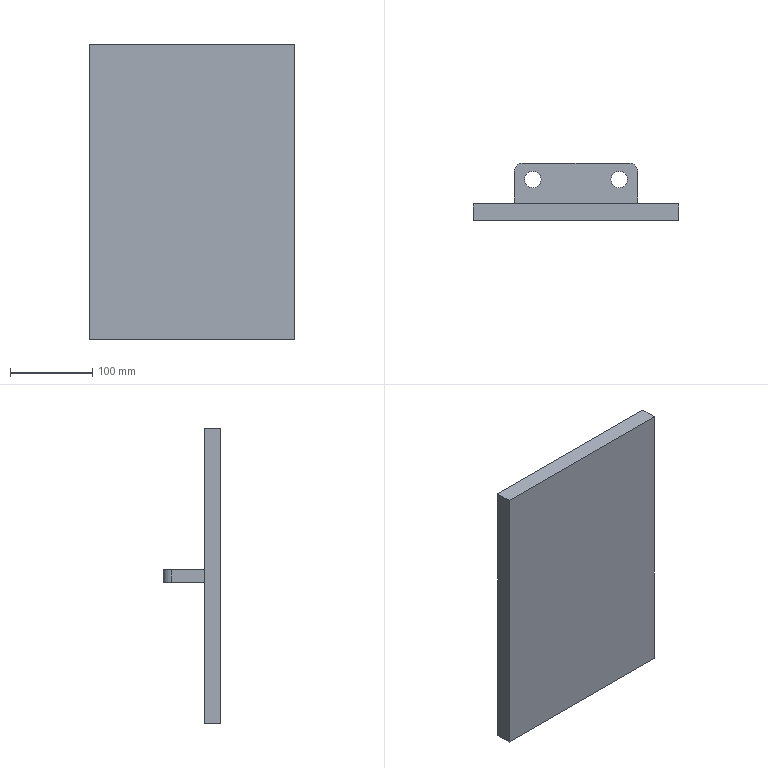Part | SolidWorks | features Cut 1, Extrusion 1, Fillet 1, ICE 1 | 1 solid | 17 faces | box 250 x 70 x 360 mm | volume 1902431 mm3 | plane 11 | cylinder 6 | commonest cylinder face diameters 20 x6
STEP:
#1=CARTESIAN_POINT('',(42.5,50.,-7.5));
#2=VERTEX_POINT('',#1);
#3=CARTESIAN_POINT('',(62.5,50.,-7.5));
#4=VERTEX_POINT('',#3);
#5=CARTESIAN_POINT('',(52.5,50.,-7.5));
#6=DIRECTION('',(0.,0.,1.));
#7=DIRECTION('',(1.,0.,0.));
#8=AXIS2_PLACEMENT_3D('',#5,#6,#7);
#9=CIRCLE('',#8,10.);
#10=EDGE_CURVE('',#2,#4,#9,.T.);
#11=ORIENTED_EDGE('',*,*,#10,.F.);
#12=CARTESIAN_POINT('',(42.5,50.,7.5));
#13=VERTEX_POINT('',#12);
#14=CARTESIAN_POINT('',(42.5,50.,-180.));
#15=DIRECTION('',(0.,0.,1.));
#16=VECTOR('',#15,1000.);
#17=LINE('',#14,#16);
#18=EDGE_CURVE('',#2,#13,#17,.T.);
#19=ORIENTED_EDGE('',*,*,#18,.T.);
#20=CARTESIAN_POINT('',(62.5,50.,7.5));
#21=VERTEX_POINT('',#20);
#22=CARTESIAN_POINT('',(52.5,50.,7.5));
#23=DIRECTION('',(0.,0.,1.));
#24=DIRECTION('',(1.,0.,0.));
#25=AXIS2_PLACEMENT_3D('',#22,#23,#24);
#26=CIRCLE('',#25,10.);
#27=EDGE_CURVE('',#13,#21,#26,.T.);
#28=ORIENTED_EDGE('',*,*,#27,.T.);
#29=CARTESIAN_POINT('',(62.5,50.,-180.));
#30=DIRECTION('',(0.,0.,1.));
#31=VECTOR('',#30,1000.);
#32=LINE('',#29,#31);
#33=EDGE_CURVE('',#4,#21,#32,.T.);
#34=ORIENTED_EDGE('',*,*,#33,.F.);
#35=EDGE_LOOP('',(#11,#19,#28,#34));
#36=FACE_OUTER_BOUND('',#35,.T.);
#37=CARTESIAN_POINT('',(52.5,50.,-180.));
#38=DIRECTION('',(0.,0.,1.));
#39=DIRECTION('',(1.,0.,0.));
#40=AXIS2_PLACEMENT_3D('',#37,#38,#39);
#41=CYLINDRICAL_SURFACE('',#40,10.);
#42=ADVANCED_FACE('',(#36),#41,.F.);
#43=CARTESIAN_POINT('',(-62.5,50.,-7.5));
#44=VERTEX_POINT('',#43);
#45=CARTESIAN_POINT('',(-42.5,50.,-7.5));
#46=VERTEX_POINT('',#45);
#47=CARTESIAN_POINT('',(-52.5,50.,-7.5));
#48=DIRECTION('',(0.,0.,1.));
#49=DIRECTION('',(1.,0.,0.));
#50=AXIS2_PLACEMENT_3D('',#47,#48,#49);
#51=CIRCLE('',#50,10.);
#52=EDGE_CURVE('',#44,#46,#51,.T.);
#53=ORIENTED_EDGE('',*,*,#52,.F.);
#54=CARTESIAN_POINT('',(-62.5,50.,7.5));
#55=VERTEX_POINT('',#54);
#56=CARTESIAN_POINT('',(-62.5,50.,-180.));
#57=DIRECTION('',(0.,0.,1.));
#58=VECTOR('',#57,1000.);
#59=LINE('',#56,#58);
#60=EDGE_CURVE('',#44,#55,#59,.T.);
#61=ORIENTED_EDGE('',*,*,#60,.T.);
#62=CARTESIAN_POINT('',(-42.5,50.,7.5));
#63=VERTEX_POINT('',#62);
#64=CARTESIAN_POINT('',(-52.5,50.,7.5));
#65=DIRECTION('',(0.,0.,1.));
#66=DIRECTION('',(-1.,0.,0.));
#67=AXIS2_PLACEMENT_3D('',#64,#65,#66);
#68=CIRCLE('',#67,10.);
#69=EDGE_CURVE('',#55,#63,#68,.T.);
#70=ORIENTED_EDGE('',*,*,#69,.T.);
#71=CARTESIAN_POINT('',(-42.5,50.,-180.));
#72=DIRECTION('',(0.,0.,1.));
#73=VECTOR('',#72,1000.);
#74=LINE('',#71,#73);
#75=EDGE_CURVE('',#46,#63,#74,.T.);
#76=ORIENTED_EDGE('',*,*,#75,.F.);
#77=EDGE_LOOP('',(#53,#61,#70,#76));
#78=FACE_OUTER_BOUND('',#77,.T.);
#79=CARTESIAN_POINT('',(-52.5,50.,-180.));
#80=DIRECTION('',(0.,0.,1.));
#81=DIRECTION('',(1.,0.,0.));
#82=AXIS2_PLACEMENT_3D('',#79,#80,#81);
#83=CYLINDRICAL_SURFACE('',#82,10.);
#84=ADVANCED_FACE('',(#78),#83,.F.);
#85=CARTESIAN_POINT('',(125.,20.,180.));
#86=VERTEX_POINT('',#85);
#87=CARTESIAN_POINT('',(125.,20.,-180.));
#88=VERTEX_POINT('',#87);
#89=CARTESIAN_POINT('',(125.,20.,-180.));
#90=DIRECTION('',(0.,0.,-1.));
#91=VECTOR('',#90,1000.);
#92=LINE('',#89,#91);
#93=EDGE_CURVE('',#86,#88,#92,.T.);
#94=ORIENTED_EDGE('',*,*,#93,.T.);
#95=CARTESIAN_POINT('',(-125.,20.,-180.));
#96=VERTEX_POINT('',#95);
#97=CARTESIAN_POINT('',(-125.,20.,-180.));
#98=DIRECTION('',(-1.,0.,0.));
#99=VECTOR('',#98,1000.);
#100=LINE('',#97,#99);
#101=EDGE_CURVE('',#88,#96,#100,.T.);
#102=ORIENTED_EDGE('',*,*,#101,.T.);
#103=CARTESIAN_POINT('',(-125.,20.,180.));
#104=VERTEX_POINT('',#103);
#105=CARTESIAN_POINT('',(-125.,20.,-180.));
#106=DIRECTION('',(0.,0.,1.));
#107=VECTOR('',#106,1000.);
#108=LINE('',#105,#107);
#109=EDGE_CURVE('',#96,#104,#108,.T.);
#110=ORIENTED_EDGE('',*,*,#109,.T.);
#111=CARTESIAN_POINT('',(-125.,20.,180.));
#112=DIRECTION('',(1.,0.,0.));
#113=VECTOR('',#112,1000.);
#114=LINE('',#111,#113);
#115=EDGE_CURVE('',#104,#86,#114,.T.);
#116=ORIENTED_EDGE('',*,*,#115,.T.);
#117=EDGE_LOOP('',(#94,#102,#110,#116));
#118=FACE_OUTER_BOUND('',#117,.T.);
#119=CARTESIAN_POINT('',(-75.,20.,7.5));
#120=VERTEX_POINT('',#119);
#121=CARTESIAN_POINT('',(75.,20.,7.5));
#122=VERTEX_POINT('',#121);
#123=CARTESIAN_POINT('',(75.,20.,7.5));
#124=DIRECTION('',(1.,0.,0.));
#125=VECTOR('',#124,1000.);
#126=LINE('',#123,#125);
#127=EDGE_CURVE('',#120,#122,#126,.T.);
#128=ORIENTED_EDGE('',*,*,#127,.F.);
#129=CARTESIAN_POINT('',(-75.,20.,-7.5));
#130=VERTEX_POINT('',#129);
#131=CARTESIAN_POINT('',(-75.,20.,-7.5));
#132=DIRECTION('',(0.,0.,1.));
#133=VECTOR('',#132,1000.);
#134=LINE('',#131,#133);
#135=EDGE_CURVE('',#130,#120,#134,.T.);
#136=ORIENTED_EDGE('',*,*,#135,.F.);
#137=CARTESIAN_POINT('',(75.,20.,-7.5));
#138=VERTEX_POINT('',#137);
#139=CARTESIAN_POINT('',(75.,20.,-7.5));
#140=DIRECTION('',(-1.,0.,0.));
#141=VECTOR('',#140,1000.);
#142=LINE('',#139,#141);
#143=EDGE_CURVE('',#138,#130,#142,.T.);
#144=ORIENTED_EDGE('',*,*,#143,.F.);
#145=CARTESIAN_POINT('',(75.,20.,-7.5));
#146=DIRECTION('',(0.,0.,-1.));
#147=VECTOR('',#146,1000.);
#148=LINE('',#145,#147);
#149=EDGE_CURVE('',#122,#138,#148,.T.);
#150=ORIENTED_EDGE('',*,*,#149,.F.);
#151=EDGE_LOOP('',(#128,#136,#144,#150));
#152=FACE_BOUND('',#151,.T.);
#153=CARTESIAN_POINT('',(0.,20.,0.));
#154=DIRECTION('',(0.,1.,0.));
#155=DIRECTION('',(0.,0.,1.));
#156=AXIS2_PLACEMENT_3D('',#153,#154,#155);
#157=PLANE('',#156);
#158=ADVANCED_FACE('',(#118,#152),#157,.T.);
#159=CARTESIAN_POINT('',(125.,0.,180.));
#160=VERTEX_POINT('',#159);
#161=CARTESIAN_POINT('',(125.,0.,-180.));
#162=VERTEX_POINT('',#161);
#163=CARTESIAN_POINT('',(125.,0.,-180.));
#164=DIRECTION('',(0.,0.,-1.));
#165=VECTOR('',#164,1000.);
#166=LINE('',#163,#165);
#167=EDGE_CURVE('',#160,#162,#166,.T.);
#168=ORIENTED_EDGE('',*,*,#167,.T.);
#169=CARTESIAN_POINT('',(125.,20.,-180.));
#170=DIRECTION('',(0.,-1.,0.));
#171=VECTOR('',#170,1000.);
#172=LINE('',#169,#171);
#173=EDGE_CURVE('',#88,#162,#172,.T.);
#174=ORIENTED_EDGE('',*,*,#173,.F.);
#175=ORIENTED_EDGE('',*,*,#93,.F.);
#176=CARTESIAN_POINT('',(125.,20.,180.));
#177=DIRECTION('',(0.,-1.,0.));
#178=VECTOR('',#177,1000.);
#179=LINE('',#176,#178);
#180=EDGE_CURVE('',#86,#160,#179,.T.);
#181=ORIENTED_EDGE('',*,*,#180,.T.);
#182=EDGE_LOOP('',(#168,#174,#175,#181));
#183=FACE_OUTER_BOUND('',#182,.T.);
#184=CARTESIAN_POINT('',(125.,20.,-180.));
#185=DIRECTION('',(-1.,0.,0.));
#186=DIRECTION('',(0.,0.,1.));
#187=AXIS2_PLACEMENT_3D('',#184,#185,#186);
#188=PLANE('',#187);
#189=ADVANCED_FACE('',(#183),#188,.F.);
#190=CARTESIAN_POINT('',(-125.,0.,-180.));
#191=VERTEX_POINT('',#190);
#192=CARTESIAN_POINT('',(-125.,0.,-180.));
#193=DIRECTION('',(-1.,0.,0.));
#194=VECTOR('',#193,1000.);
#195=LINE('',#192,#194);
#196=EDGE_CURVE('',#162,#191,#195,.T.);
#197=ORIENTED_EDGE('',*,*,#196,.T.);
#198=CARTESIAN_POINT('',(-125.,20.,-180.));
#199=DIRECTION('',(0.,-1.,0.));
#200=VECTOR('',#199,1000.);
#201=LINE('',#198,#200);
#202=EDGE_CURVE('',#96,#191,#201,.T.);
#203=ORIENTED_EDGE('',*,*,#202,.F.);
#204=ORIENTED_EDGE('',*,*,#101,.F.);
#205=ORIENTED_EDGE('',*,*,#173,.T.);
#206=EDGE_LOOP('',(#197,#203,#204,#205));
#207=FACE_OUTER_BOUND('',#206,.T.);
#208=CARTESIAN_POINT('',(-125.,20.,-180.));
#209=DIRECTION('',(0.,0.,1.));
#210=DIRECTION('',(1.,0.,0.));
#211=AXIS2_PLACEMENT_3D('',#208,#209,#210);
#212=PLANE('',#211);
#213=ADVANCED_FACE('',(#207),#212,.F.);
#214=CARTESIAN_POINT('',(-125.,0.,180.));
#215=VERTEX_POINT('',#214);
#216=CARTESIAN_POINT('',(-125.,0.,-180.));
#217=DIRECTION('',(0.,0.,1.));
#218=VECTOR('',#217,1000.);
#219=LINE('',#216,#218);
#220=EDGE_CURVE('',#191,#215,#219,.T.);
#221=ORIENTED_EDGE('',*,*,#220,.T.);
#222=CARTESIAN_POINT('',(-125.,20.,180.));
#223=DIRECTION('',(0.,-1.,0.));
#224=VECTOR('',#223,1000.);
#225=LINE('',#222,#224);
#226=EDGE_CURVE('',#104,#215,#225,.T.);
#227=ORIENTED_EDGE('',*,*,#226,.F.);
#228=ORIENTED_EDGE('',*,*,#109,.F.);
#229=ORIENTED_EDGE('',*,*,#202,.T.);
#230=EDGE_LOOP('',(#221,#227,#228,#229));
#231=FACE_OUTER_BOUND('',#230,.T.);
#232=CARTESIAN_POINT('',(-125.,20.,-180.));
#233=DIRECTION('',(1.,0.,0.));
#234=DIRECTION('',(0.,0.,-1.));
#235=AXIS2_PLACEMENT_3D('',#232,#233,#234);
#236=PLANE('',#235);
#237=ADVANCED_FACE('',(#231),#236,.F.);
#238=CARTESIAN_POINT('',(-125.,0.,180.));
#239=DIRECTION('',(1.,0.,0.));
#240=VECTOR('',#239,1000.);
#241=LINE('',#238,#240);
#242=EDGE_CURVE('',#215,#160,#241,.T.);
#243=ORIENTED_EDGE('',*,*,#242,.T.);
#244=ORIENTED_EDGE('',*,*,#180,.F.);
#245=ORIENTED_EDGE('',*,*,#115,.F.);
#246=ORIENTED_EDGE('',*,*,#226,.T.);
#247=EDGE_LOOP('',(#243,#244,#245,#246));
#248=FACE_OUTER_BOUND('',#247,.T.);
#249=CARTESIAN_POINT('',(-125.,20.,180.));
#250=DIRECTION('',(0.,0.,-1.));
#251=DIRECTION('',(-1.,0.,0.));
#252=AXIS2_PLACEMENT_3D('',#249,#250,#251);
#253=PLANE('',#252);
#254=ADVANCED_FACE('',(#248),#253,.F.);
#255=ORIENTED_EDGE('',*,*,#167,.F.);
#256=ORIENTED_EDGE('',*,*,#242,.F.);
#257=ORIENTED_EDGE('',*,*,#220,.F.);
#258=ORIENTED_EDGE('',*,*,#196,.F.);
#259=EDGE_LOOP('',(#255,#256,#257,#258));
#260=FACE_OUTER_BOUND('',#259,.T.);
#261=CARTESIAN_POINT('',(0.,0.,0.));
#262=DIRECTION('',(0.,1.,0.));
#263=DIRECTION('',(0.,0.,1.));
#264=AXIS2_PLACEMENT_3D('',#261,#262,#263);
#265=PLANE('',#264);
#266=ADVANCED_FACE('',(#260),#265,.F.);
#267=CARTESIAN_POINT('',(-75.,60.,7.5));
#268=VERTEX_POINT('',#267);
#269=CARTESIAN_POINT('',(-75.,70.,7.5));
#270=DIRECTION('',(0.,-1.,0.));
#271=VECTOR('',#270,1000.);
#272=LINE('',#269,#271);
#273=EDGE_CURVE('',#268,#120,#272,.T.);
#274=ORIENTED_EDGE('',*,*,#273,.F.);
#275=CARTESIAN_POINT('',(-75.,60.,-7.5));
#276=VERTEX_POINT('',#275);
#277=CARTESIAN_POINT('',(-75.,60.,-7.5));
#278=DIRECTION('',(0.,0.,-1.));
#279=VECTOR('',#278,1000.);
#280=LINE('',#277,#279);
#281=EDGE_CURVE('',#268,#276,#280,.T.);
#282=ORIENTED_EDGE('',*,*,#281,.T.);
#283=CARTESIAN_POINT('',(-75.,70.,-7.5));
#284=DIRECTION('',(0.,-1.,0.));
#285=VECTOR('',#284,1000.);
#286=LINE('',#283,#285);
#287=EDGE_CURVE('',#276,#130,#286,.T.);
#288=ORIENTED_EDGE('',*,*,#287,.T.);
#289=ORIENTED_EDGE('',*,*,#135,.T.);
#290=EDGE_LOOP('',(#274,#282,#288,#289));
#291=FACE_OUTER_BOUND('',#290,.T.);
#292=CARTESIAN_POINT('',(-75.,70.,-7.5));
#293=DIRECTION('',(1.,0.,0.));
#294=DIRECTION('',(0.,0.,-1.));
#295=AXIS2_PLACEMENT_3D('',#292,#293,#294);
#296=PLANE('',#295);
#297=ADVANCED_FACE('',(#291),#296,.F.);
#298=CARTESIAN_POINT('',(52.5,50.,7.5));
#299=DIRECTION('',(0.,0.,1.));
#300=DIRECTION('',(1.,0.,0.));
#301=AXIS2_PLACEMENT_3D('',#298,#299,#300);
#302=CIRCLE('',#301,10.);
#303=EDGE_CURVE('',#21,#13,#302,.T.);
#304=ORIENTED_EDGE('',*,*,#303,.F.);
#305=ORIENTED_EDGE('',*,*,#27,.F.);
#306=EDGE_LOOP('',(#304,#305));
#307=FACE_BOUND('',#306,.T.);
#308=CARTESIAN_POINT('',(-52.5,50.,7.5));
#309=DIRECTION('',(0.,0.,1.));
#310=DIRECTION('',(-1.,0.,0.));
#311=AXIS2_PLACEMENT_3D('',#308,#309,#310);
#312=CIRCLE('',#311,10.);
#313=EDGE_CURVE('',#63,#55,#312,.T.);
#314=ORIENTED_EDGE('',*,*,#313,.F.);
#315=ORIENTED_EDGE('',*,*,#69,.F.);
#316=EDGE_LOOP('',(#314,#315));
#317=FACE_BOUND('',#316,.T.);
#318=CARTESIAN_POINT('',(-65.,70.,7.5));
#319=VERTEX_POINT('',#318);
#320=CARTESIAN_POINT('',(65.,70.,7.5));
#321=VERTEX_POINT('',#320);
#322=CARTESIAN_POINT('',(75.,70.,7.5));
#323=DIRECTION('',(1.,0.,0.));
#324=VECTOR('',#323,1000.);
#325=LINE('',#322,#324);
#326=EDGE_CURVE('',#319,#321,#325,.T.);
#327=ORIENTED_EDGE('',*,*,#326,.F.);
#328=CARTESIAN_POINT('',(-65.,60.,7.5));
#329=DIRECTION('',(0.,0.,1.));
#330=DIRECTION('',(-1.,0.,0.));
#331=AXIS2_PLACEMENT_3D('',#328,#329,#330);
#332=CIRCLE('',#331,10.);
#333=EDGE_CURVE('',#319,#268,#332,.T.);
#334=ORIENTED_EDGE('',*,*,#333,.T.);
#335=ORIENTED_EDGE('',*,*,#273,.T.);
#336=ORIENTED_EDGE('',*,*,#127,.T.);
#337=CARTESIAN_POINT('',(75.,60.,7.5));
#338=VERTEX_POINT('',#337);
#339=CARTESIAN_POINT('',(75.,70.,7.5));
#340=DIRECTION('',(0.,-1.,0.));
#341=VECTOR('',#340,1000.);
#342=LINE('',#339,#341);
#343=EDGE_CURVE('',#338,#122,#342,.T.);
#344=ORIENTED_EDGE('',*,*,#343,.F.);
#345=CARTESIAN_POINT('',(65.,60.,7.5));
#346=DIRECTION('',(0.,0.,1.));
#347=DIRECTION('',(-1.,0.,0.));
#348=AXIS2_PLACEMENT_3D('',#345,#346,#347);
#349=CIRCLE('',#348,10.);
#350=EDGE_CURVE('',#338,#321,#349,.T.);
#351=ORIENTED_EDGE('',*,*,#350,.T.);
#352=EDGE_LOOP('',(#327,#334,#335,#336,#344,#351));
#353=FACE_OUTER_BOUND('',#352,.T.);
#354=CARTESIAN_POINT('',(75.,70.,7.5));
#355=DIRECTION('',(0.,0.,-1.));
#356=DIRECTION('',(-1.,0.,0.));
#357=AXIS2_PLACEMENT_3D('',#354,#355,#356);
#358=PLANE('',#357);
#359=ADVANCED_FACE('',(#307,#317,#353),#358,.F.);
#360=CARTESIAN_POINT('',(75.,60.,-7.5));
#361=VERTEX_POINT('',#360);
#362=CARTESIAN_POINT('',(75.,70.,-7.5));
#363=DIRECTION('',(0.,-1.,0.));
#364=VECTOR('',#363,1000.);
#365=LINE('',#362,#364);
#366=EDGE_CURVE('',#361,#138,#365,.T.);
#367=ORIENTED_EDGE('',*,*,#366,.F.);
#368=CARTESIAN_POINT('',(75.,60.,-7.5));
#369=DIRECTION('',(0.,0.,1.));
#370=VECTOR('',#369,1000.);
#371=LINE('',#368,#370);
#372=EDGE_CURVE('',#361,#338,#371,.T.);
#373=ORIENTED_EDGE('',*,*,#372,.T.);
#374=ORIENTED_EDGE('',*,*,#343,.T.);
#375=ORIENTED_EDGE('',*,*,#149,.T.);
#376=EDGE_LOOP('',(#367,#373,#374,#375));
#377=FACE_OUTER_BOUND('',#376,.T.);
#378=CARTESIAN_POINT('',(75.,70.,-7.5));
#379=DIRECTION('',(-1.,0.,0.));
#380=DIRECTION('',(0.,0.,1.));
#381=AXIS2_PLACEMENT_3D('',#378,#379,#380);
#382=PLANE('',#381);
#383=ADVANCED_FACE('',(#377),#382,.F.);
#384=CARTESIAN_POINT('',(52.5,50.,-7.5));
#385=DIRECTION('',(0.,0.,1.));
#386=DIRECTION('',(1.,0.,0.));
#387=AXIS2_PLACEMENT_3D('',#384,#385,#386);
#388=CIRCLE('',#387,10.);
#389=EDGE_CURVE('',#4,#2,#388,.T.);
#390=ORIENTED_EDGE('',*,*,#389,.T.);
#391=ORIENTED_EDGE('',*,*,#10,.T.);
#392=EDGE_LOOP('',(#390,#391));
#393=FACE_BOUND('',#392,.T.);
#394=CARTESIAN_POINT('',(-52.5,50.,-7.5));
#395=DIRECTION('',(0.,0.,1.));
#396=DIRECTION('',(1.,0.,0.));
#397=AXIS2_PLACEMENT_3D('',#394,#395,#396);
#398=CIRCLE('',#397,10.);
#399=EDGE_CURVE('',#46,#44,#398,.T.);
#400=ORIENTED_EDGE('',*,*,#399,.T.);
#401=ORIENTED_EDGE('',*,*,#52,.T.);
#402=EDGE_LOOP('',(#400,#401));
#403=FACE_BOUND('',#402,.T.);
#404=ORIENTED_EDGE('',*,*,#287,.F.);
#405=CARTESIAN_POINT('',(-65.,70.,-7.5));
#406=VERTEX_POINT('',#405);
#407=CARTESIAN_POINT('',(-65.,60.,-7.5));
#408=DIRECTION('',(0.,0.,-1.));
#409=DIRECTION('',(1.,0.,0.));
#410=AXIS2_PLACEMENT_3D('',#407,#408,#409);
#411=CIRCLE('',#410,10.);
#412=EDGE_CURVE('',#276,#406,#411,.T.);
#413=ORIENTED_EDGE('',*,*,#412,.T.);
#414=CARTESIAN_POINT('',(65.,70.,-7.5));
#415=VERTEX_POINT('',#414);
#416=CARTESIAN_POINT('',(75.,70.,-7.5));
#417=DIRECTION('',(-1.,0.,0.));
#418=VECTOR('',#417,1000.);
#419=LINE('',#416,#418);
#420=EDGE_CURVE('',#415,#406,#419,.T.);
#421=ORIENTED_EDGE('',*,*,#420,.F.);
#422=CARTESIAN_POINT('',(65.,60.,-7.5));
#423=DIRECTION('',(0.,0.,-1.));
#424=DIRECTION('',(1.,0.,0.));
#425=AXIS2_PLACEMENT_3D('',#422,#423,#424);
#426=CIRCLE('',#425,10.);
#427=EDGE_CURVE('',#415,#361,#426,.T.);
#428=ORIENTED_EDGE('',*,*,#427,.T.);
#429=ORIENTED_EDGE('',*,*,#366,.T.);
#430=ORIENTED_EDGE('',*,*,#143,.T.);
#431=EDGE_LOOP('',(#404,#413,#421,#428,#429,#430));
#432=FACE_OUTER_BOUND('',#431,.T.);
#433=CARTESIAN_POINT('',(75.,70.,-7.5));
#434=DIRECTION('',(0.,0.,1.));
#435=DIRECTION('',(1.,0.,0.));
#436=AXIS2_PLACEMENT_3D('',#433,#434,#435);
#437=PLANE('',#436);
#438=ADVANCED_FACE('',(#393,#403,#432),#437,.F.);
#439=ORIENTED_EDGE('',*,*,#420,.T.);
#440=CARTESIAN_POINT('',(-65.,70.,0.));
#441=DIRECTION('',(0.,0.,1.));
#442=VECTOR('',#441,1000.);
#443=LINE('',#440,#442);
#444=EDGE_CURVE('',#406,#319,#443,.T.);
#445=ORIENTED_EDGE('',*,*,#444,.T.);
#446=ORIENTED_EDGE('',*,*,#326,.T.);
#447=CARTESIAN_POINT('',(65.,70.,0.));
#448=DIRECTION('',(0.,0.,-1.));
#449=VECTOR('',#448,1000.);
#450=LINE('',#447,#449);
#451=EDGE_CURVE('',#321,#415,#450,.T.);
#452=ORIENTED_EDGE('',*,*,#451,.T.);
#453=EDGE_LOOP('',(#439,#445,#446,#452));
#454=FACE_OUTER_BOUND('',#453,.T.);
#455=CARTESIAN_POINT('',(0.,70.,0.));
#456=DIRECTION('',(0.,-1.,0.));
#457=DIRECTION('',(0.,0.,-1.));
#458=AXIS2_PLACEMENT_3D('',#455,#456,#457);
#459=PLANE('',#458);
#460=ADVANCED_FACE('',(#454),#459,.F.);
#461=ORIENTED_EDGE('',*,*,#412,.F.);
#462=ORIENTED_EDGE('',*,*,#281,.F.);
#463=ORIENTED_EDGE('',*,*,#333,.F.);
#464=ORIENTED_EDGE('',*,*,#444,.F.);
#465=EDGE_LOOP('',(#461,#462,#463,#464));
#466=FACE_OUTER_BOUND('',#465,.T.);
#467=CARTESIAN_POINT('',(-65.,60.,0.));
#468=DIRECTION('',(0.,0.,1.));
#469=DIRECTION('',(1.,0.,0.));
#470=AXIS2_PLACEMENT_3D('',#467,#468,#469);
#471=CYLINDRICAL_SURFACE('',#470,10.);
#472=ADVANCED_FACE('',(#466),#471,.T.);
#473=ORIENTED_EDGE('',*,*,#350,.F.);
#474=ORIENTED_EDGE('',*,*,#372,.F.);
#475=ORIENTED_EDGE('',*,*,#427,.F.);
#476=ORIENTED_EDGE('',*,*,#451,.F.);
#477=EDGE_LOOP('',(#473,#474,#475,#476));
#478=FACE_OUTER_BOUND('',#477,.T.);
#479=CARTESIAN_POINT('',(65.,60.,0.));
#480=DIRECTION('',(0.,0.,-1.));
#481=DIRECTION('',(-1.,0.,0.));
#482=AXIS2_PLACEMENT_3D('',#479,#480,#481);
#483=CYLINDRICAL_SURFACE('',#482,10.);
#484=ADVANCED_FACE('',(#478),#483,.T.);
#485=ORIENTED_EDGE('',*,*,#60,.F.);
#486=ORIENTED_EDGE('',*,*,#399,.F.);
#487=ORIENTED_EDGE('',*,*,#75,.T.);
#488=ORIENTED_EDGE('',*,*,#313,.T.);
#489=EDGE_LOOP('',(#485,#486,#487,#488));
#490=FACE_OUTER_BOUND('',#489,.T.);
#491=CARTESIAN_POINT('',(-52.5,50.,-180.));
#492=DIRECTION('',(0.,0.,1.));
#493=DIRECTION('',(1.,0.,0.));
#494=AXIS2_PLACEMENT_3D('',#491,#492,#493);
#495=CYLINDRICAL_SURFACE('',#494,10.);
#496=ADVANCED_FACE('',(#490),#495,.F.);
#497=ORIENTED_EDGE('',*,*,#18,.F.);
#498=ORIENTED_EDGE('',*,*,#389,.F.);
#499=ORIENTED_EDGE('',*,*,#33,.T.);
#500=ORIENTED_EDGE('',*,*,#303,.T.);
#501=EDGE_LOOP('',(#497,#498,#499,#500));
#502=FACE_OUTER_BOUND('',#501,.T.);
#503=CARTESIAN_POINT('',(52.5,50.,-180.));
#504=DIRECTION('',(0.,0.,1.));
#505=DIRECTION('',(1.,0.,0.));
#506=AXIS2_PLACEMENT_3D('',#503,#504,#505);
#507=CYLINDRICAL_SURFACE('',#506,10.);
#508=ADVANCED_FACE('',(#502),#507,.F.);
#509=CLOSED_SHELL('',(#42,#84,#158,#189,#213,#237,#254,#266,#297,#359,#383,#438,#460,#472,#484,#496,#508));
#510=MANIFOLD_SOLID_BREP('',#509);
#511=CARTESIAN_POINT('',(0.,0.,0.));
#512=DIRECTION('',(0.,0.,1.));
#513=DIRECTION('',(1.,0.,0.));
#514=AXIS2_PLACEMENT_3D('',#511,#512,#513);
#515=(LENGTH_UNIT()NAMED_UNIT(*)SI_UNIT(.MILLI.,.METRE.));
#516=UNCERTAINTY_MEASURE_WITH_UNIT(LENGTH_MEASURE(0.00001),#515,'','');
#517=(NAMED_UNIT(*)PLANE_ANGLE_UNIT()SI_UNIT($,.RADIAN.));
#518=(NAMED_UNIT(*)SI_UNIT($,.STERADIAN.)SOLID_ANGLE_UNIT());
#519=(GEOMETRIC_REPRESENTATION_CONTEXT(3)GLOBAL_UNCERTAINTY_ASSIGNED_CONTEXT((#516))GLOBAL_UNIT_ASSIGNED_CONTEXT((#515,#517,#518))REPRESENTATION_CONTEXT('',''));
#520=ADVANCED_BREP_SHAPE_REPRESENTATION('',(#510,#514),#519);